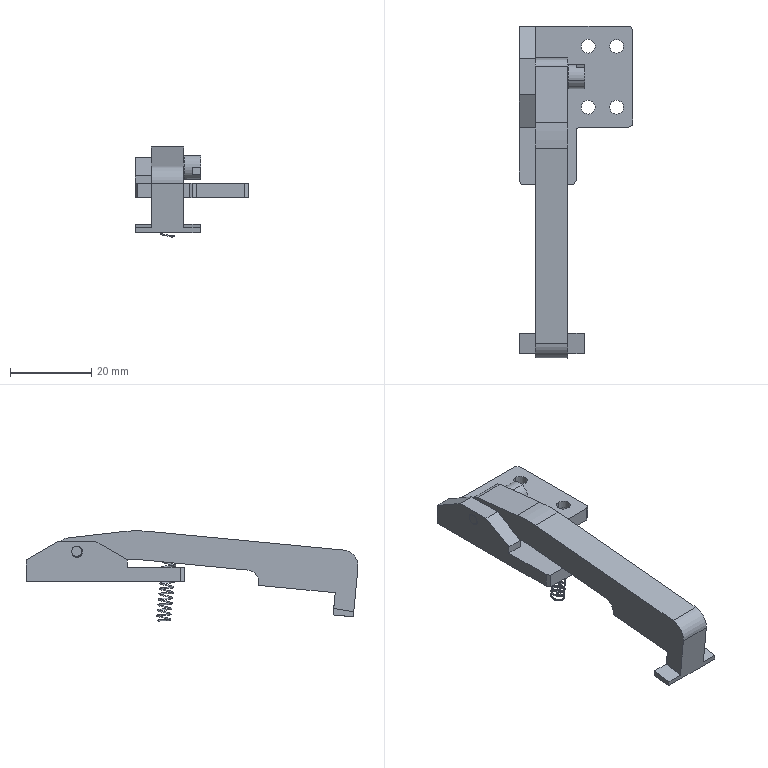Part | NX | features BREP 5 | 4 solids | 122 faces | box 28 x 81.879 x 22.282 mm | volume 7199 mm3 | plane 55 | cylinder 55 | cone 8 | spline 4 | commonest cylinder face diameters 3 x18 6 x9 3.4 x8 4.5 x7 2.5 x4 5 x4